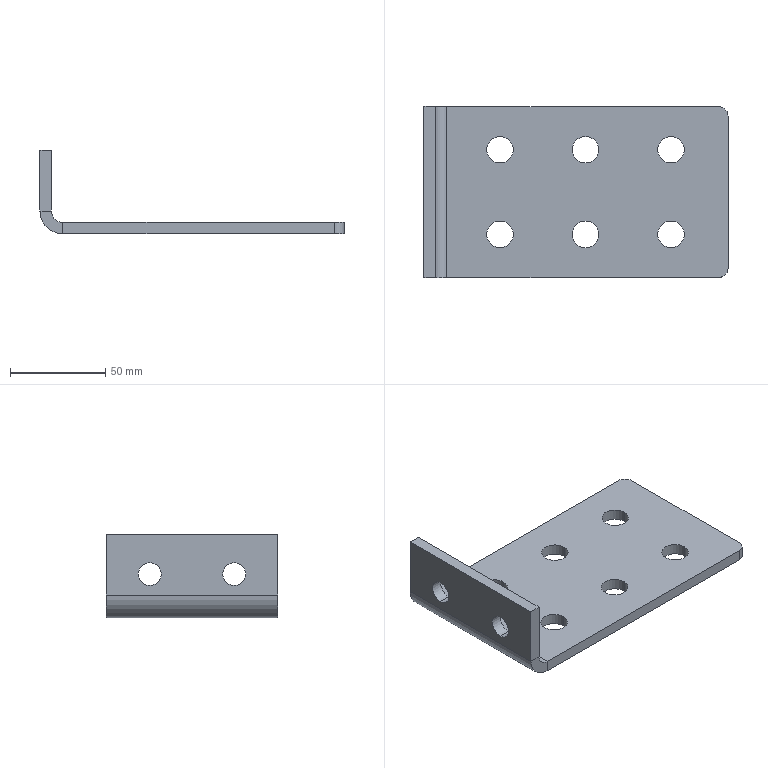Part | STEP file | 64728105 | 1 solid | 32 faces | box 160 x 90 x 44 mm | volume 97871 mm3 | cylinder 20 | plane 12 | commonest cylinder face diameters 14 x12 12 x5 10 x2 24 x1